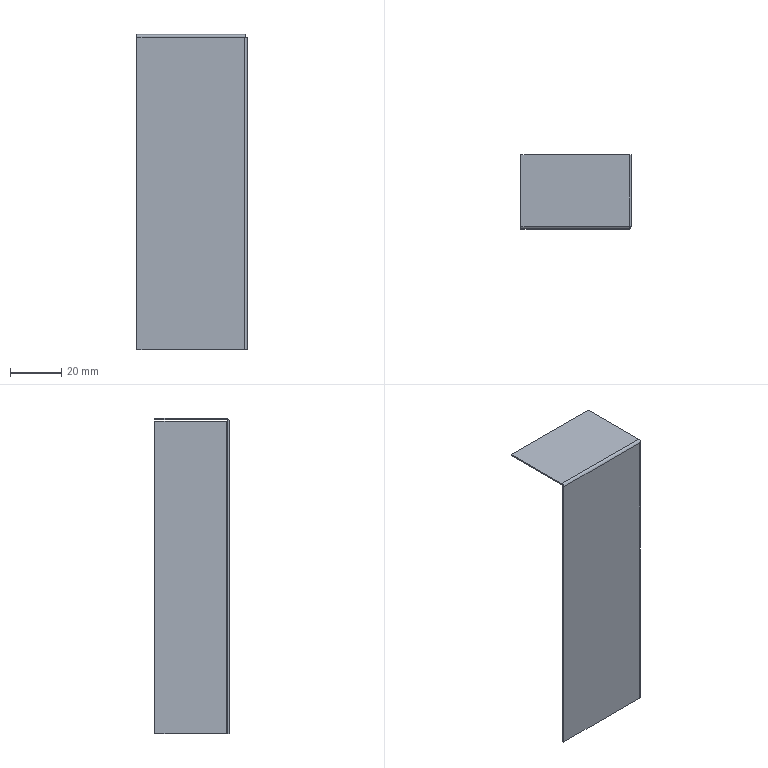Part | SolidWorks | features BaseBody 1 | 1 solid | 17 faces | box 42.935 x 28.935 x 122.935 mm | volume 4950 mm3 | plane 13 | cylinder 4 | commonest cylinder face diameters 1 x2 2 x2
STEP:
#1=CARTESIAN_POINT('',(-75.314,45.987,-0.5));
#2=VERTEX_POINT('',#1);
#3=CARTESIAN_POINT('',(-75.314,45.987,-122.435));
#4=VERTEX_POINT('',#3);
#5=CARTESIAN_POINT('',(-75.314,45.987,-61.185));
#6=DIRECTION('',(0.,0.,-1.));
#7=VECTOR('',#6,1000.);
#8=LINE('',#5,#7);
#9=EDGE_CURVE('',#2,#4,#8,.T.);
#10=ORIENTED_EDGE('',*,*,#9,.T.);
#11=CARTESIAN_POINT('',(-33.379,45.987,-122.435));
#12=VERTEX_POINT('',#11);
#13=CARTESIAN_POINT('',(-54.064,45.987,-122.435));
#14=DIRECTION('',(1.,0.,0.));
#15=VECTOR('',#14,1000.);
#16=LINE('',#13,#15);
#17=EDGE_CURVE('',#4,#12,#16,.T.);
#18=ORIENTED_EDGE('',*,*,#17,.T.);
#19=CARTESIAN_POINT('',(-33.379,45.987,-0.5));
#20=VERTEX_POINT('',#19);
#21=CARTESIAN_POINT('',(-33.379,45.987,-61.185));
#22=DIRECTION('',(0.,0.,1.));
#23=VECTOR('',#22,1000.);
#24=LINE('',#21,#23);
#25=EDGE_CURVE('',#12,#20,#24,.T.);
#26=ORIENTED_EDGE('',*,*,#25,.T.);
#27=CARTESIAN_POINT('',(-54.064,45.987,-0.5));
#28=DIRECTION('',(-1.,0.,0.));
#29=VECTOR('',#28,1000.);
#30=LINE('',#27,#29);
#31=EDGE_CURVE('',#20,#2,#30,.T.);
#32=ORIENTED_EDGE('',*,*,#31,.T.);
#33=EDGE_LOOP('',(#10,#18,#26,#32));
#34=FACE_OUTER_BOUND('',#33,.T.);
#35=CARTESIAN_POINT('',(-54.064,45.987,-61.185));
#36=DIRECTION('',(0.,-1.,0.));
#37=DIRECTION('',(0.,0.,-1.));
#38=AXIS2_PLACEMENT_3D('',#35,#36,#37);
#39=PLANE('',#38);
#40=ADVANCED_FACE('',(#34),#39,.T.);
#41=CARTESIAN_POINT('',(-75.314,46.487,-122.435));
#42=VERTEX_POINT('',#41);
#43=CARTESIAN_POINT('',(-75.314,46.487,-122.435));
#44=DIRECTION('',(0.,1.,0.));
#45=VECTOR('',#44,1000.);
#46=LINE('',#43,#45);
#47=EDGE_CURVE('',#4,#42,#46,.T.);
#48=ORIENTED_EDGE('',*,*,#47,.T.);
#49=CARTESIAN_POINT('',(-33.379,46.487,-122.435));
#50=VERTEX_POINT('',#49);
#51=CARTESIAN_POINT('',(-32.814,46.487,-122.435));
#52=DIRECTION('',(1.,0.,0.));
#53=VECTOR('',#52,1000.);
#54=LINE('',#51,#53);
#55=EDGE_CURVE('',#42,#50,#54,.T.);
#56=ORIENTED_EDGE('',*,*,#55,.T.);
#57=CARTESIAN_POINT('',(-32.879,46.987,-122.435));
#58=VERTEX_POINT('',#57);
#59=CARTESIAN_POINT('',(-33.379,46.987,-122.435));
#60=DIRECTION('',(0.,0.,1.));
#61=DIRECTION('',(-1.,0.,0.));
#62=AXIS2_PLACEMENT_3D('',#59,#60,#61);
#63=CIRCLE('',#62,0.5);
#64=EDGE_CURVE('',#50,#58,#63,.T.);
#65=ORIENTED_EDGE('',*,*,#64,.T.);
#66=CARTESIAN_POINT('',(-32.879,74.922,-122.435));
#67=VERTEX_POINT('',#66);
#68=CARTESIAN_POINT('',(-32.879,46.422,-122.435));
#69=DIRECTION('',(0.,1.,0.));
#70=VECTOR('',#69,1000.);
#71=LINE('',#68,#70);
#72=EDGE_CURVE('',#58,#67,#71,.T.);
#73=ORIENTED_EDGE('',*,*,#72,.T.);
#74=CARTESIAN_POINT('',(-32.379,74.922,-122.435));
#75=VERTEX_POINT('',#74);
#76=CARTESIAN_POINT('',(-32.879,74.922,-122.435));
#77=DIRECTION('',(-1.,0.,0.));
#78=VECTOR('',#77,1000.);
#79=LINE('',#76,#78);
#80=EDGE_CURVE('',#75,#67,#79,.T.);
#81=ORIENTED_EDGE('',*,*,#80,.F.);
#82=CARTESIAN_POINT('',(-32.379,46.987,-122.435));
#83=VERTEX_POINT('',#82);
#84=CARTESIAN_POINT('',(-32.379,25.172,-122.435));
#85=DIRECTION('',(0.,1.,0.));
#86=VECTOR('',#85,1000.);
#87=LINE('',#84,#86);
#88=EDGE_CURVE('',#83,#75,#87,.T.);
#89=ORIENTED_EDGE('',*,*,#88,.F.);
#90=CARTESIAN_POINT('',(-33.379,46.987,-122.435));
#91=DIRECTION('',(0.,0.,1.));
#92=DIRECTION('',(-1.,0.,0.));
#93=AXIS2_PLACEMENT_3D('',#90,#91,#92);
#94=CIRCLE('',#93,1.);
#95=EDGE_CURVE('',#12,#83,#94,.T.);
#96=ORIENTED_EDGE('',*,*,#95,.F.);
#97=ORIENTED_EDGE('',*,*,#17,.F.);
#98=EDGE_LOOP('',(#48,#56,#65,#73,#81,#89,#96,#97));
#99=FACE_OUTER_BOUND('',#98,.T.);
#100=CARTESIAN_POINT('',(-32.814,46.487,-122.435));
#101=DIRECTION('',(0.,0.,-1.));
#102=DIRECTION('',(-1.,0.,0.));
#103=AXIS2_PLACEMENT_3D('',#100,#101,#102);
#104=PLANE('',#103);
#105=ADVANCED_FACE('',(#99),#104,.T.);
#106=ORIENTED_EDGE('',*,*,#47,.F.);
#107=ORIENTED_EDGE('',*,*,#9,.F.);
#108=CARTESIAN_POINT('',(-75.314,46.987,0.5));
#109=VERTEX_POINT('',#108);
#110=CARTESIAN_POINT('',(-75.314,46.987,-0.5));
#111=DIRECTION('',(1.,0.,0.));
#112=DIRECTION('',(0.,0.,-1.));
#113=AXIS2_PLACEMENT_3D('',#110,#111,#112);
#114=CIRCLE('',#113,1.);
#115=EDGE_CURVE('',#109,#2,#114,.T.);
#116=ORIENTED_EDGE('',*,*,#115,.F.);
#117=CARTESIAN_POINT('',(-75.314,74.922,0.5));
#118=VERTEX_POINT('',#117);
#119=CARTESIAN_POINT('',(-75.314,-14.828,0.5));
#120=DIRECTION('',(0.,-1.,0.));
#121=VECTOR('',#120,1000.);
#122=LINE('',#119,#121);
#123=EDGE_CURVE('',#118,#109,#122,.T.);
#124=ORIENTED_EDGE('',*,*,#123,.F.);
#125=CARTESIAN_POINT('',(-75.314,74.922,0.));
#126=VERTEX_POINT('',#125);
#127=CARTESIAN_POINT('',(-75.314,74.922,0.));
#128=DIRECTION('',(0.,0.,-1.));
#129=VECTOR('',#128,1000.);
#130=LINE('',#127,#129);
#131=EDGE_CURVE('',#118,#126,#130,.T.);
#132=ORIENTED_EDGE('',*,*,#131,.T.);
#133=CARTESIAN_POINT('',(-75.314,46.987,0.));
#134=VERTEX_POINT('',#133);
#135=CARTESIAN_POINT('',(-75.314,-76.078,0.));
#136=DIRECTION('',(0.,-1.,0.));
#137=VECTOR('',#136,1000.);
#138=LINE('',#135,#137);
#139=EDGE_CURVE('',#126,#134,#138,.T.);
#140=ORIENTED_EDGE('',*,*,#139,.T.);
#141=CARTESIAN_POINT('',(-75.314,46.487,-0.5));
#142=VERTEX_POINT('',#141);
#143=CARTESIAN_POINT('',(-75.314,46.987,-0.5));
#144=DIRECTION('',(1.,0.,0.));
#145=DIRECTION('',(0.,0.,-1.));
#146=AXIS2_PLACEMENT_3D('',#143,#144,#145);
#147=CIRCLE('',#146,0.5);
#148=EDGE_CURVE('',#134,#142,#147,.T.);
#149=ORIENTED_EDGE('',*,*,#148,.T.);
#150=CARTESIAN_POINT('',(-75.314,46.487,-122.435));
#151=DIRECTION('',(0.,0.,-1.));
#152=VECTOR('',#151,1000.);
#153=LINE('',#150,#152);
#154=EDGE_CURVE('',#142,#42,#153,.T.);
#155=ORIENTED_EDGE('',*,*,#154,.T.);
#156=EDGE_LOOP('',(#106,#107,#116,#124,#132,#140,#149,#155));
#157=FACE_OUTER_BOUND('',#156,.T.);
#158=CARTESIAN_POINT('',(-75.314,46.487,-122.435));
#159=DIRECTION('',(-1.,0.,0.));
#160=DIRECTION('',(0.,0.,1.));
#161=AXIS2_PLACEMENT_3D('',#158,#159,#160);
#162=PLANE('',#161);
#163=ADVANCED_FACE('',(#157),#162,.T.);
#164=CARTESIAN_POINT('',(-32.814,45.987,-0.5));
#165=VERTEX_POINT('',#164);
#166=CARTESIAN_POINT('',(-32.814,46.987,0.5));
#167=VERTEX_POINT('',#166);
#168=CARTESIAN_POINT('',(-32.814,46.987,-0.5));
#169=DIRECTION('',(-1.,0.,0.));
#170=DIRECTION('',(0.,0.,-1.));
#171=AXIS2_PLACEMENT_3D('',#168,#169,#170);
#172=CIRCLE('',#171,1.);
#173=EDGE_CURVE('',#165,#167,#172,.T.);
#174=ORIENTED_EDGE('',*,*,#173,.T.);
#175=CARTESIAN_POINT('',(-54.064,46.987,0.5));
#176=DIRECTION('',(-1.,0.,0.));
#177=VECTOR('',#176,1000.);
#178=LINE('',#175,#177);
#179=EDGE_CURVE('',#167,#109,#178,.T.);
#180=ORIENTED_EDGE('',*,*,#179,.T.);
#181=ORIENTED_EDGE('',*,*,#115,.T.);
#182=ORIENTED_EDGE('',*,*,#31,.F.);
#183=CARTESIAN_POINT('',(-54.064,45.987,-0.5));
#184=DIRECTION('',(1.,0.,0.));
#185=VECTOR('',#184,1000.);
#186=LINE('',#183,#185);
#187=EDGE_CURVE('',#20,#165,#186,.T.);
#188=ORIENTED_EDGE('',*,*,#187,.T.);
#189=EDGE_LOOP('',(#174,#180,#181,#182,#188));
#190=FACE_OUTER_BOUND('',#189,.T.);
#191=CARTESIAN_POINT('',(-54.064,46.987,-0.5));
#192=DIRECTION('',(1.,0.,0.));
#193=DIRECTION('',(0.,0.,-1.));
#194=AXIS2_PLACEMENT_3D('',#191,#192,#193);
#195=CYLINDRICAL_SURFACE('',#194,1.);
#196=ADVANCED_FACE('',(#190),#195,.T.);
#197=ORIENTED_EDGE('',*,*,#95,.T.);
#198=CARTESIAN_POINT('',(-32.379,46.987,-0.5));
#199=VERTEX_POINT('',#198);
#200=CARTESIAN_POINT('',(-32.379,46.987,-61.467));
#201=DIRECTION('',(0.,0.,1.));
#202=VECTOR('',#201,1000.);
#203=LINE('',#200,#202);
#204=EDGE_CURVE('',#83,#199,#203,.T.);
#205=ORIENTED_EDGE('',*,*,#204,.T.);
#206=CARTESIAN_POINT('',(-32.814,46.162,-0.5));
#207=VERTEX_POINT('',#206);
#208=CARTESIAN_POINT('',(-33.379,46.987,-0.5));
#209=DIRECTION('',(0.,0.,-1.));
#210=DIRECTION('',(-1.,0.,0.));
#211=AXIS2_PLACEMENT_3D('',#208,#209,#210);
#212=CIRCLE('',#211,1.);
#213=EDGE_CURVE('',#199,#207,#212,.T.);
#214=ORIENTED_EDGE('',*,*,#213,.T.);
#215=CARTESIAN_POINT('',(-33.379,46.987,-0.5));
#216=DIRECTION('',(0.,0.,-1.));
#217=DIRECTION('',(-1.,0.,0.));
#218=AXIS2_PLACEMENT_3D('',#215,#216,#217);
#219=CIRCLE('',#218,1.);
#220=EDGE_CURVE('',#207,#20,#219,.T.);
#221=ORIENTED_EDGE('',*,*,#220,.T.);
#222=ORIENTED_EDGE('',*,*,#25,.F.);
#223=EDGE_LOOP('',(#197,#205,#214,#221,#222));
#224=FACE_OUTER_BOUND('',#223,.T.);
#225=CARTESIAN_POINT('',(-33.379,46.987,-61.467));
#226=DIRECTION('',(0.,0.,-1.));
#227=DIRECTION('',(-1.,0.,0.));
#228=AXIS2_PLACEMENT_3D('',#225,#226,#227);
#229=CYLINDRICAL_SURFACE('',#228,1.);
#230=ADVANCED_FACE('',(#224),#229,.T.);
#231=ORIENTED_EDGE('',*,*,#55,.F.);
#232=ORIENTED_EDGE('',*,*,#154,.F.);
#233=CARTESIAN_POINT('',(-33.379,46.487,-0.5));
#234=VERTEX_POINT('',#233);
#235=CARTESIAN_POINT('',(-54.064,46.487,-0.5));
#236=DIRECTION('',(-1.,0.,0.));
#237=VECTOR('',#236,1000.);
#238=LINE('',#235,#237);
#239=EDGE_CURVE('',#234,#142,#238,.T.);
#240=ORIENTED_EDGE('',*,*,#239,.F.);
#241=CARTESIAN_POINT('',(-33.379,46.487,-61.185));
#242=DIRECTION('',(0.,0.,1.));
#243=VECTOR('',#242,1000.);
#244=LINE('',#241,#243);
#245=EDGE_CURVE('',#50,#234,#244,.T.);
#246=ORIENTED_EDGE('',*,*,#245,.F.);
#247=EDGE_LOOP('',(#231,#232,#240,#246));
#248=FACE_OUTER_BOUND('',#247,.T.);
#249=CARTESIAN_POINT('',(-54.064,46.487,-61.185));
#250=DIRECTION('',(0.,-1.,0.));
#251=DIRECTION('',(0.,0.,-1.));
#252=AXIS2_PLACEMENT_3D('',#249,#250,#251);
#253=PLANE('',#252);
#254=ADVANCED_FACE('',(#248),#253,.F.);
#255=CARTESIAN_POINT('',(-32.814,74.922,0.5));
#256=VERTEX_POINT('',#255);
#257=CARTESIAN_POINT('',(-54.064,74.922,0.5));
#258=DIRECTION('',(-1.,0.,0.));
#259=VECTOR('',#258,1000.);
#260=LINE('',#257,#259);
#261=EDGE_CURVE('',#256,#118,#260,.T.);
#262=ORIENTED_EDGE('',*,*,#261,.T.);
#263=ORIENTED_EDGE('',*,*,#123,.T.);
#264=ORIENTED_EDGE('',*,*,#179,.F.);
#265=CARTESIAN_POINT('',(-32.814,-14.828,0.5));
#266=DIRECTION('',(0.,1.,0.));
#267=VECTOR('',#266,1000.);
#268=LINE('',#265,#267);
#269=EDGE_CURVE('',#167,#256,#268,.T.);
#270=ORIENTED_EDGE('',*,*,#269,.T.);
#271=EDGE_LOOP('',(#262,#263,#264,#270));
#272=FACE_OUTER_BOUND('',#271,.T.);
#273=CARTESIAN_POINT('',(-54.064,-14.828,0.5));
#274=DIRECTION('',(0.,0.,1.));
#275=DIRECTION('',(1.,0.,0.));
#276=AXIS2_PLACEMENT_3D('',#273,#274,#275);
#277=PLANE('',#276);
#278=ADVANCED_FACE('',(#272),#277,.T.);
#279=CARTESIAN_POINT('',(-32.814,46.487,-0.5));
#280=VERTEX_POINT('',#279);
#281=CARTESIAN_POINT('',(-32.814,46.987,0.));
#282=VERTEX_POINT('',#281);
#283=CARTESIAN_POINT('',(-32.814,46.987,-0.5));
#284=DIRECTION('',(-1.,0.,0.));
#285=DIRECTION('',(0.,0.,-1.));
#286=AXIS2_PLACEMENT_3D('',#283,#284,#285);
#287=CIRCLE('',#286,0.5);
#288=EDGE_CURVE('',#280,#282,#287,.T.);
#289=ORIENTED_EDGE('',*,*,#288,.T.);
#290=CARTESIAN_POINT('',(-32.814,74.922,0.));
#291=VERTEX_POINT('',#290);
#292=CARTESIAN_POINT('',(-32.814,46.422,0.));
#293=DIRECTION('',(0.,1.,0.));
#294=VECTOR('',#293,1000.);
#295=LINE('',#292,#294);
#296=EDGE_CURVE('',#282,#291,#295,.T.);
#297=ORIENTED_EDGE('',*,*,#296,.T.);
#298=CARTESIAN_POINT('',(-32.814,74.922,0.));
#299=DIRECTION('',(0.,0.,-1.));
#300=VECTOR('',#299,1000.);
#301=LINE('',#298,#300);
#302=EDGE_CURVE('',#256,#291,#301,.T.);
#303=ORIENTED_EDGE('',*,*,#302,.F.);
#304=ORIENTED_EDGE('',*,*,#269,.F.);
#305=ORIENTED_EDGE('',*,*,#173,.F.);
#306=CARTESIAN_POINT('',(-32.814,46.987,-0.5));
#307=DIRECTION('',(0.,1.,0.));
#308=VECTOR('',#307,1000.);
#309=LINE('',#306,#308);
#310=EDGE_CURVE('',#165,#207,#309,.T.);
#311=ORIENTED_EDGE('',*,*,#310,.T.);
#312=CARTESIAN_POINT('',(-32.814,46.987,-0.5));
#313=DIRECTION('',(0.,1.,0.));
#314=VECTOR('',#313,1000.);
#315=LINE('',#312,#314);
#316=EDGE_CURVE('',#207,#280,#315,.T.);
#317=ORIENTED_EDGE('',*,*,#316,.T.);
#318=EDGE_LOOP('',(#289,#297,#303,#304,#305,#311,#317));
#319=FACE_OUTER_BOUND('',#318,.T.);
#320=CARTESIAN_POINT('',(-32.814,46.987,1.375));
#321=DIRECTION('',(1.,0.,0.));
#322=DIRECTION('',(0.,0.,-1.));
#323=AXIS2_PLACEMENT_3D('',#320,#321,#322);
#324=PLANE('',#323);
#325=ADVANCED_FACE('',(#319),#324,.T.);
#326=ORIENTED_EDGE('',*,*,#310,.F.);
#327=ORIENTED_EDGE('',*,*,#187,.F.);
#328=ORIENTED_EDGE('',*,*,#220,.F.);
#329=EDGE_LOOP('',(#326,#327,#328));
#330=FACE_OUTER_BOUND('',#329,.T.);
#331=CARTESIAN_POINT('',(-33.379,46.487,-0.5));
#332=DIRECTION('',(0.,0.,1.));
#333=DIRECTION('',(1.,0.,0.));
#334=AXIS2_PLACEMENT_3D('',#331,#332,#333);
#335=PLANE('',#334);
#336=ADVANCED_FACE('',(#330),#335,.F.);
#337=CARTESIAN_POINT('',(-32.379,74.922,-0.5));
#338=VERTEX_POINT('',#337);
#339=CARTESIAN_POINT('',(-32.379,74.922,-61.185));
#340=DIRECTION('',(0.,0.,1.));
#341=VECTOR('',#340,1000.);
#342=LINE('',#339,#341);
#343=EDGE_CURVE('',#75,#338,#342,.T.);
#344=ORIENTED_EDGE('',*,*,#343,.T.);
#345=CARTESIAN_POINT('',(-32.379,25.172,-0.5));
#346=DIRECTION('',(0.,-1.,0.));
#347=VECTOR('',#346,1000.);
#348=LINE('',#345,#347);
#349=EDGE_CURVE('',#338,#199,#348,.T.);
#350=ORIENTED_EDGE('',*,*,#349,.T.);
#351=ORIENTED_EDGE('',*,*,#204,.F.);
#352=ORIENTED_EDGE('',*,*,#88,.T.);
#353=EDGE_LOOP('',(#344,#350,#351,#352));
#354=FACE_OUTER_BOUND('',#353,.T.);
#355=CARTESIAN_POINT('',(-32.379,25.172,-61.185));
#356=DIRECTION('',(1.,0.,0.));
#357=DIRECTION('',(0.,0.,-1.));
#358=AXIS2_PLACEMENT_3D('',#355,#356,#357);
#359=PLANE('',#358);
#360=ADVANCED_FACE('',(#354),#359,.T.);
#361=ORIENTED_EDGE('',*,*,#213,.F.);
#362=ORIENTED_EDGE('',*,*,#349,.F.);
#363=CARTESIAN_POINT('',(-32.879,74.922,-0.5));
#364=VERTEX_POINT('',#363);
#365=CARTESIAN_POINT('',(-32.879,74.922,-0.5));
#366=DIRECTION('',(-1.,0.,0.));
#367=VECTOR('',#366,1000.);
#368=LINE('',#365,#367);
#369=EDGE_CURVE('',#338,#364,#368,.T.);
#370=ORIENTED_EDGE('',*,*,#369,.T.);
#371=CARTESIAN_POINT('',(-32.879,46.987,-0.5));
#372=VERTEX_POINT('',#371);
#373=CARTESIAN_POINT('',(-32.879,46.422,-0.5));
#374=DIRECTION('',(0.,-1.,0.));
#375=VECTOR('',#374,1000.);
#376=LINE('',#373,#375);
#377=EDGE_CURVE('',#364,#372,#376,.T.);
#378=ORIENTED_EDGE('',*,*,#377,.T.);
#379=CARTESIAN_POINT('',(-33.379,46.987,-0.5));
#380=DIRECTION('',(0.,0.,-1.));
#381=DIRECTION('',(-1.,0.,0.));
#382=AXIS2_PLACEMENT_3D('',#379,#380,#381);
#383=CIRCLE('',#382,0.5);
#384=EDGE_CURVE('',#372,#234,#383,.T.);
#385=ORIENTED_EDGE('',*,*,#384,.T.);
#386=CARTESIAN_POINT('',(-33.379,46.487,-0.5));
#387=DIRECTION('',(1.,0.,0.));
#388=VECTOR('',#387,1000.);
#389=LINE('',#386,#388);
#390=EDGE_CURVE('',#234,#280,#389,.T.);
#391=ORIENTED_EDGE('',*,*,#390,.T.);
#392=ORIENTED_EDGE('',*,*,#316,.F.);
#393=EDGE_LOOP('',(#361,#362,#370,#378,#385,#391,#392));
#394=FACE_OUTER_BOUND('',#393,.T.);
#395=CARTESIAN_POINT('',(-33.379,45.112,-0.5));
#396=DIRECTION('',(0.,0.,1.));
#397=DIRECTION('',(1.,0.,0.));
#398=AXIS2_PLACEMENT_3D('',#395,#396,#397);
#399=PLANE('',#398);
#400=ADVANCED_FACE('',(#394),#399,.T.);
#401=CARTESIAN_POINT('',(-32.879,46.987,-61.467));
#402=DIRECTION('',(0.,0.,1.));
#403=VECTOR('',#402,1000.);
#404=LINE('',#401,#403);
#405=EDGE_CURVE('',#58,#372,#404,.T.);
#406=ORIENTED_EDGE('',*,*,#405,.F.);
#407=ORIENTED_EDGE('',*,*,#64,.F.);
#408=ORIENTED_EDGE('',*,*,#245,.T.);
#409=ORIENTED_EDGE('',*,*,#384,.F.);
#410=EDGE_LOOP('',(#406,#407,#408,#409));
#411=FACE_OUTER_BOUND('',#410,.T.);
#412=CARTESIAN_POINT('',(-33.379,46.987,-61.467));
#413=DIRECTION('',(0.,0.,-1.));
#414=DIRECTION('',(-1.,0.,0.));
#415=AXIS2_PLACEMENT_3D('',#412,#413,#414);
#416=CYLINDRICAL_SURFACE('',#415,0.5);
#417=ADVANCED_FACE('',(#411),#416,.F.);
#418=CARTESIAN_POINT('',(-54.064,46.987,0.));
#419=DIRECTION('',(-1.,0.,0.));
#420=VECTOR('',#419,1000.);
#421=LINE('',#418,#420);
#422=EDGE_CURVE('',#282,#134,#421,.T.);
#423=ORIENTED_EDGE('',*,*,#422,.F.);
#424=ORIENTED_EDGE('',*,*,#288,.F.);
#425=ORIENTED_EDGE('',*,*,#390,.F.);
#426=ORIENTED_EDGE('',*,*,#239,.T.);
#427=ORIENTED_EDGE('',*,*,#148,.F.);
#428=EDGE_LOOP('',(#423,#424,#425,#426,#427));
#429=FACE_OUTER_BOUND('',#428,.T.);
#430=CARTESIAN_POINT('',(-54.064,46.987,-0.5));
#431=DIRECTION('',(1.,0.,0.));
#432=DIRECTION('',(0.,0.,-1.));
#433=AXIS2_PLACEMENT_3D('',#430,#431,#432);
#434=CYLINDRICAL_SURFACE('',#433,0.5);
#435=ADVANCED_FACE('',(#429),#434,.F.);
#436=CARTESIAN_POINT('',(-75.314,74.922,0.));
#437=DIRECTION('',(-1.,0.,0.));
#438=VECTOR('',#437,1000.);
#439=LINE('',#436,#438);
#440=EDGE_CURVE('',#291,#126,#439,.T.);
#441=ORIENTED_EDGE('',*,*,#440,.T.);
#442=ORIENTED_EDGE('',*,*,#131,.F.);
#443=ORIENTED_EDGE('',*,*,#261,.F.);
#444=ORIENTED_EDGE('',*,*,#302,.T.);
#445=EDGE_LOOP('',(#441,#442,#443,#444));
#446=FACE_OUTER_BOUND('',#445,.T.);
#447=CARTESIAN_POINT('',(-75.314,74.922,0.));
#448=DIRECTION('',(0.,1.,0.));
#449=DIRECTION('',(0.,0.,1.));
#450=AXIS2_PLACEMENT_3D('',#447,#448,#449);
#451=PLANE('',#450);
#452=ADVANCED_FACE('',(#446),#451,.T.);
#453=CARTESIAN_POINT('',(-32.879,74.922,-0.5));
#454=DIRECTION('',(0.,0.,1.));
#455=VECTOR('',#454,1000.);
#456=LINE('',#453,#455);
#457=EDGE_CURVE('',#67,#364,#456,.T.);
#458=ORIENTED_EDGE('',*,*,#457,.T.);
#459=ORIENTED_EDGE('',*,*,#369,.F.);
#460=ORIENTED_EDGE('',*,*,#343,.F.);
#461=ORIENTED_EDGE('',*,*,#80,.T.);
#462=EDGE_LOOP('',(#458,#459,#460,#461));
#463=FACE_OUTER_BOUND('',#462,.T.);
#464=CARTESIAN_POINT('',(-32.879,74.922,-0.5));
#465=DIRECTION('',(0.,1.,0.));
#466=DIRECTION('',(0.,0.,1.));
#467=AXIS2_PLACEMENT_3D('',#464,#465,#466);
#468=PLANE('',#467);
#469=ADVANCED_FACE('',(#463),#468,.T.);
#470=ORIENTED_EDGE('',*,*,#377,.F.);
#471=ORIENTED_EDGE('',*,*,#457,.F.);
#472=ORIENTED_EDGE('',*,*,#72,.F.);
#473=ORIENTED_EDGE('',*,*,#405,.T.);
#474=EDGE_LOOP('',(#470,#471,#472,#473));
#475=FACE_OUTER_BOUND('',#474,.T.);
#476=CARTESIAN_POINT('',(-32.879,25.172,-61.185));
#477=DIRECTION('',(1.,0.,0.));
#478=DIRECTION('',(0.,0.,-1.));
#479=AXIS2_PLACEMENT_3D('',#476,#477,#478);
#480=PLANE('',#479);
#481=ADVANCED_FACE('',(#475),#480,.F.);
#482=ORIENTED_EDGE('',*,*,#139,.F.);
#483=ORIENTED_EDGE('',*,*,#440,.F.);
#484=ORIENTED_EDGE('',*,*,#296,.F.);
#485=ORIENTED_EDGE('',*,*,#422,.T.);
#486=EDGE_LOOP('',(#482,#483,#484,#485));
#487=FACE_OUTER_BOUND('',#486,.T.);
#488=CARTESIAN_POINT('',(-54.064,-14.828,0.));
#489=DIRECTION('',(0.,0.,1.));
#490=DIRECTION('',(1.,0.,0.));
#491=AXIS2_PLACEMENT_3D('',#488,#489,#490);
#492=PLANE('',#491);
#493=ADVANCED_FACE('',(#487),#492,.F.);
#494=CLOSED_SHELL('',(#40,#105,#163,#196,#230,#254,#278,#325,#336,#360,#400,#417,#435,#452,#469,#481,#493));
#495=MANIFOLD_SOLID_BREP('',#494);
#496=CARTESIAN_POINT('',(0.,0.,0.));
#497=DIRECTION('',(0.,0.,1.));
#498=DIRECTION('',(1.,0.,0.));
#499=AXIS2_PLACEMENT_3D('',#496,#497,#498);
#500=(LENGTH_UNIT()NAMED_UNIT(*)SI_UNIT(.MILLI.,.METRE.));
#501=UNCERTAINTY_MEASURE_WITH_UNIT(LENGTH_MEASURE(0.00001),#500,'','');
#502=(NAMED_UNIT(*)PLANE_ANGLE_UNIT()SI_UNIT($,.RADIAN.));
#503=(NAMED_UNIT(*)SI_UNIT($,.STERADIAN.)SOLID_ANGLE_UNIT());
#504=(GEOMETRIC_REPRESENTATION_CONTEXT(3)GLOBAL_UNCERTAINTY_ASSIGNED_CONTEXT((#501))GLOBAL_UNIT_ASSIGNED_CONTEXT((#500,#502,#503))REPRESENTATION_CONTEXT('',''));
#505=ADVANCED_BREP_SHAPE_REPRESENTATION('',(#495,#499),#504);